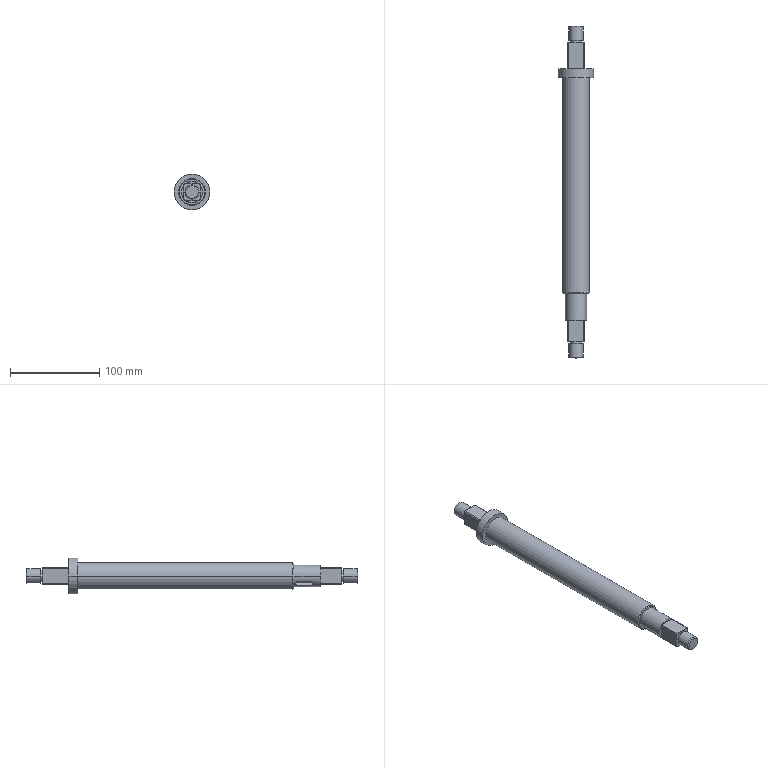Part | SolidWorks | features MirrorStock 1 | 1 solid | 50 faces | box 40 x 372 x 40 mm | volume 221068 mm3 | plane 24 | cylinder 20 | cone 6 | commonest cylinder face diameters 24 x6 13 x4 16 x4 6 x2 30 x2 40 x2
STEP:
#1=CARTESIAN_POINT('',(-7.,-186.,0.));
#2=VERTEX_POINT('',#1);
#3=CARTESIAN_POINT('',(7.,-186.,0.));
#4=VERTEX_POINT('',#3);
#5=CARTESIAN_POINT('',(0.,-186.,0.));
#6=DIRECTION('',(0.,1.,0.));
#7=DIRECTION('',(-1.,0.,0.));
#8=AXIS2_PLACEMENT_3D('',#5,#6,#7);
#9=CIRCLE('',#8,7.);
#10=EDGE_CURVE('',#2,#4,#9,.T.);
#11=ORIENTED_EDGE('',*,*,#10,.T.);
#12=CARTESIAN_POINT('',(8.,-185.,0.));
#13=VERTEX_POINT('',#12);
#14=CARTESIAN_POINT('',(7.,-186.,0.));
#15=DIRECTION('',(0.7071,0.7071,0.));
#16=VECTOR('',#15,1000.);
#17=LINE('',#14,#16);
#18=EDGE_CURVE('',#4,#13,#17,.T.);
#19=ORIENTED_EDGE('',*,*,#18,.T.);
#20=CARTESIAN_POINT('',(-8.,-185.,0.));
#21=VERTEX_POINT('',#20);
#22=CARTESIAN_POINT('',(0.,-185.,0.));
#23=DIRECTION('',(0.,-1.,0.));
#24=DIRECTION('',(-1.,0.,0.));
#25=AXIS2_PLACEMENT_3D('',#22,#23,#24);
#26=CIRCLE('',#25,8.);
#27=EDGE_CURVE('',#13,#21,#26,.T.);
#28=ORIENTED_EDGE('',*,*,#27,.T.);
#29=CARTESIAN_POINT('',(-7.,-186.,0.));
#30=DIRECTION('',(-0.7071,0.7071,0.));
#31=VECTOR('',#30,1000.);
#32=LINE('',#29,#31);
#33=EDGE_CURVE('',#2,#21,#32,.T.);
#34=ORIENTED_EDGE('',*,*,#33,.F.);
#35=EDGE_LOOP('',(#11,#19,#28,#34));
#36=FACE_OUTER_BOUND('',#35,.T.);
#37=CARTESIAN_POINT('',(0.,-186.,0.));
#38=DIRECTION('',(0.,1.,0.));
#39=DIRECTION('',(-1.,0.,0.));
#40=AXIS2_PLACEMENT_3D('',#37,#38,#39);
#41=CONICAL_SURFACE('',#40,7.,0.7854);
#42=ADVANCED_FACE('',(#36),#41,.T.);
#43=CARTESIAN_POINT('',(-14.,-114.,0.));
#44=VERTEX_POINT('',#43);
#45=CARTESIAN_POINT('',(14.,-114.,0.));
#46=VERTEX_POINT('',#45);
#47=CARTESIAN_POINT('',(0.,-114.,0.));
#48=DIRECTION('',(0.,1.,0.));
#49=DIRECTION('',(-1.,0.,0.));
#50=AXIS2_PLACEMENT_3D('',#47,#48,#49);
#51=CIRCLE('',#50,14.);
#52=EDGE_CURVE('',#44,#46,#51,.T.);
#53=ORIENTED_EDGE('',*,*,#52,.T.);
#54=CARTESIAN_POINT('',(15.,-113.,0.));
#55=VERTEX_POINT('',#54);
#56=CARTESIAN_POINT('',(14.,-114.,0.));
#57=DIRECTION('',(0.7071,0.7071,0.));
#58=VECTOR('',#57,1000.);
#59=LINE('',#56,#58);
#60=EDGE_CURVE('',#46,#55,#59,.T.);
#61=ORIENTED_EDGE('',*,*,#60,.T.);
#62=CARTESIAN_POINT('',(-15.,-113.,0.));
#63=VERTEX_POINT('',#62);
#64=CARTESIAN_POINT('',(0.,-113.,0.));
#65=DIRECTION('',(0.,-1.,0.));
#66=DIRECTION('',(-1.,0.,0.));
#67=AXIS2_PLACEMENT_3D('',#64,#65,#66);
#68=CIRCLE('',#67,15.);
#69=EDGE_CURVE('',#55,#63,#68,.T.);
#70=ORIENTED_EDGE('',*,*,#69,.T.);
#71=CARTESIAN_POINT('',(-14.,-114.,0.));
#72=DIRECTION('',(-0.7071,0.7071,0.));
#73=VECTOR('',#72,1000.);
#74=LINE('',#71,#73);
#75=EDGE_CURVE('',#44,#63,#74,.T.);
#76=ORIENTED_EDGE('',*,*,#75,.F.);
#77=EDGE_LOOP('',(#53,#61,#70,#76));
#78=FACE_OUTER_BOUND('',#77,.T.);
#79=CARTESIAN_POINT('',(0.,-114.,0.));
#80=DIRECTION('',(0.,1.,0.));
#81=DIRECTION('',(-1.,0.,0.));
#82=AXIS2_PLACEMENT_3D('',#79,#80,#81);
#83=CONICAL_SURFACE('',#82,14.,0.7854);
#84=ADVANCED_FACE('',(#78),#83,.T.);
#85=CARTESIAN_POINT('',(7.,186.,0.));
#86=VERTEX_POINT('',#85);
#87=CARTESIAN_POINT('',(-7.,186.,0.));
#88=VERTEX_POINT('',#87);
#89=CARTESIAN_POINT('',(0.,186.,0.));
#90=DIRECTION('',(0.,-1.,0.));
#91=DIRECTION('',(1.,0.,0.));
#92=AXIS2_PLACEMENT_3D('',#89,#90,#91);
#93=CIRCLE('',#92,7.);
#94=EDGE_CURVE('',#86,#88,#93,.T.);
#95=ORIENTED_EDGE('',*,*,#94,.T.);
#96=CARTESIAN_POINT('',(-8.,185.,0.));
#97=VERTEX_POINT('',#96);
#98=CARTESIAN_POINT('',(-8.,185.,0.));
#99=DIRECTION('',(-0.7071,-0.7071,0.));
#100=VECTOR('',#99,1000.);
#101=LINE('',#98,#100);
#102=EDGE_CURVE('',#88,#97,#101,.T.);
#103=ORIENTED_EDGE('',*,*,#102,.T.);
#104=CARTESIAN_POINT('',(8.,185.,0.));
#105=VERTEX_POINT('',#104);
#106=CARTESIAN_POINT('',(0.,185.,0.));
#107=DIRECTION('',(0.,1.,0.));
#108=DIRECTION('',(1.,0.,0.));
#109=AXIS2_PLACEMENT_3D('',#106,#107,#108);
#110=CIRCLE('',#109,8.);
#111=EDGE_CURVE('',#97,#105,#110,.T.);
#112=ORIENTED_EDGE('',*,*,#111,.T.);
#113=CARTESIAN_POINT('',(8.,185.,0.));
#114=DIRECTION('',(0.7071,-0.7071,0.));
#115=VECTOR('',#114,1000.);
#116=LINE('',#113,#115);
#117=EDGE_CURVE('',#86,#105,#116,.T.);
#118=ORIENTED_EDGE('',*,*,#117,.F.);
#119=EDGE_LOOP('',(#95,#103,#112,#118));
#120=FACE_OUTER_BOUND('',#119,.T.);
#121=CARTESIAN_POINT('',(0.,185.,0.));
#122=DIRECTION('',(0.,-1.,0.));
#123=DIRECTION('',(1.,0.,0.));
#124=AXIS2_PLACEMENT_3D('',#121,#122,#123);
#125=CONICAL_SURFACE('',#124,8.,0.7854);
#126=ADVANCED_FACE('',(#120),#125,.T.);
#127=CARTESIAN_POINT('',(-8.,-170.,0.));
#128=VERTEX_POINT('',#127);
#129=CARTESIAN_POINT('',(8.,-170.,0.));
#130=VERTEX_POINT('',#129);
#131=CARTESIAN_POINT('',(0.,-170.,0.));
#132=DIRECTION('',(0.,1.,0.));
#133=DIRECTION('',(1.,0.,0.));
#134=AXIS2_PLACEMENT_3D('',#131,#132,#133);
#135=CIRCLE('',#134,8.);
#136=EDGE_CURVE('',#128,#130,#135,.T.);
#137=ORIENTED_EDGE('',*,*,#136,.F.);
#138=CARTESIAN_POINT('',(-8.,-186.,0.));
#139=DIRECTION('',(0.,-1.,0.));
#140=VECTOR('',#139,1000.);
#141=LINE('',#138,#140);
#142=EDGE_CURVE('',#128,#21,#141,.T.);
#143=ORIENTED_EDGE('',*,*,#142,.T.);
#144=ORIENTED_EDGE('',*,*,#27,.F.);
#145=CARTESIAN_POINT('',(8.,-186.,0.));
#146=DIRECTION('',(0.,-1.,0.));
#147=VECTOR('',#146,1000.);
#148=LINE('',#145,#147);
#149=EDGE_CURVE('',#130,#13,#148,.T.);
#150=ORIENTED_EDGE('',*,*,#149,.F.);
#151=EDGE_LOOP('',(#137,#143,#144,#150));
#152=FACE_OUTER_BOUND('',#151,.T.);
#153=CARTESIAN_POINT('',(0.,-186.,0.));
#154=DIRECTION('',(0.,-1.,0.));
#155=DIRECTION('',(1.,0.,0.));
#156=AXIS2_PLACEMENT_3D('',#153,#154,#155);
#157=CYLINDRICAL_SURFACE('',#156,8.);
#158=ADVANCED_FACE('',(#152),#157,.T.);
#159=CARTESIAN_POINT('',(-6.5,-168.,0.));
#160=VERTEX_POINT('',#159);
#161=CARTESIAN_POINT('',(6.5,-168.,0.));
#162=VERTEX_POINT('',#161);
#163=CARTESIAN_POINT('',(0.,-168.,0.));
#164=DIRECTION('',(0.,1.,0.));
#165=DIRECTION('',(1.,0.,0.));
#166=AXIS2_PLACEMENT_3D('',#163,#164,#165);
#167=CIRCLE('',#166,6.5);
#168=EDGE_CURVE('',#160,#162,#167,.T.);
#169=ORIENTED_EDGE('',*,*,#168,.F.);
#170=CARTESIAN_POINT('',(-6.5,-170.,0.));
#171=VERTEX_POINT('',#170);
#172=CARTESIAN_POINT('',(-6.5,-186.,0.));
#173=DIRECTION('',(0.,-1.,0.));
#174=VECTOR('',#173,1000.);
#175=LINE('',#172,#174);
#176=EDGE_CURVE('',#160,#171,#175,.T.);
#177=ORIENTED_EDGE('',*,*,#176,.T.);
#178=CARTESIAN_POINT('',(6.5,-170.,0.));
#179=VERTEX_POINT('',#178);
#180=CARTESIAN_POINT('',(0.,-170.,0.));
#181=DIRECTION('',(0.,1.,0.));
#182=DIRECTION('',(1.,0.,0.));
#183=AXIS2_PLACEMENT_3D('',#180,#181,#182);
#184=CIRCLE('',#183,6.5);
#185=EDGE_CURVE('',#171,#179,#184,.T.);
#186=ORIENTED_EDGE('',*,*,#185,.T.);
#187=CARTESIAN_POINT('',(6.5,-186.,0.));
#188=DIRECTION('',(0.,-1.,0.));
#189=VECTOR('',#188,1000.);
#190=LINE('',#187,#189);
#191=EDGE_CURVE('',#162,#179,#190,.T.);
#192=ORIENTED_EDGE('',*,*,#191,.F.);
#193=EDGE_LOOP('',(#169,#177,#186,#192));
#194=FACE_OUTER_BOUND('',#193,.T.);
#195=CARTESIAN_POINT('',(0.,-186.,0.));
#196=DIRECTION('',(0.,-1.,0.));
#197=DIRECTION('',(1.,0.,0.));
#198=AXIS2_PLACEMENT_3D('',#195,#196,#197);
#199=CYLINDRICAL_SURFACE('',#198,6.5);
#200=ADVANCED_FACE('',(#194),#199,.T.);
#201=CARTESIAN_POINT('',(-15.,128.,0.));
#202=VERTEX_POINT('',#201);
#203=CARTESIAN_POINT('',(15.,128.,0.));
#204=VERTEX_POINT('',#203);
#205=CARTESIAN_POINT('',(0.,128.,0.));
#206=DIRECTION('',(0.,1.,0.));
#207=DIRECTION('',(1.,0.,0.));
#208=AXIS2_PLACEMENT_3D('',#205,#206,#207);
#209=CIRCLE('',#208,15.);
#210=EDGE_CURVE('',#202,#204,#209,.T.);
#211=ORIENTED_EDGE('',*,*,#210,.F.);
#212=CARTESIAN_POINT('',(-15.,-186.,0.));
#213=DIRECTION('',(0.,-1.,0.));
#214=VECTOR('',#213,1000.);
#215=LINE('',#212,#214);
#216=EDGE_CURVE('',#202,#63,#215,.T.);
#217=ORIENTED_EDGE('',*,*,#216,.T.);
#218=ORIENTED_EDGE('',*,*,#69,.F.);
#219=CARTESIAN_POINT('',(15.,-186.,0.));
#220=DIRECTION('',(0.,-1.,0.));
#221=VECTOR('',#220,1000.);
#222=LINE('',#219,#221);
#223=EDGE_CURVE('',#204,#55,#222,.T.);
#224=ORIENTED_EDGE('',*,*,#223,.F.);
#225=EDGE_LOOP('',(#211,#217,#218,#224));
#226=FACE_OUTER_BOUND('',#225,.T.);
#227=CARTESIAN_POINT('',(0.,-186.,0.));
#228=DIRECTION('',(0.,-1.,0.));
#229=DIRECTION('',(1.,0.,0.));
#230=AXIS2_PLACEMENT_3D('',#227,#228,#229);
#231=CYLINDRICAL_SURFACE('',#230,15.);
#232=ADVANCED_FACE('',(#226),#231,.T.);
#233=CARTESIAN_POINT('',(-20.,138.,0.));
#234=VERTEX_POINT('',#233);
#235=CARTESIAN_POINT('',(20.,138.,0.));
#236=VERTEX_POINT('',#235);
#237=CARTESIAN_POINT('',(0.,138.,0.));
#238=DIRECTION('',(0.,1.,0.));
#239=DIRECTION('',(1.,0.,0.));
#240=AXIS2_PLACEMENT_3D('',#237,#238,#239);
#241=CIRCLE('',#240,20.);
#242=EDGE_CURVE('',#234,#236,#241,.T.);
#243=ORIENTED_EDGE('',*,*,#242,.F.);
#244=CARTESIAN_POINT('',(-20.,128.,0.));
#245=VERTEX_POINT('',#244);
#246=CARTESIAN_POINT('',(-20.,-186.,0.));
#247=DIRECTION('',(0.,-1.,0.));
#248=VECTOR('',#247,1000.);
#249=LINE('',#246,#248);
#250=EDGE_CURVE('',#234,#245,#249,.T.);
#251=ORIENTED_EDGE('',*,*,#250,.T.);
#252=CARTESIAN_POINT('',(20.,128.,0.));
#253=VERTEX_POINT('',#252);
#254=CARTESIAN_POINT('',(0.,128.,0.));
#255=DIRECTION('',(0.,1.,0.));
#256=DIRECTION('',(1.,0.,0.));
#257=AXIS2_PLACEMENT_3D('',#254,#255,#256);
#258=CIRCLE('',#257,20.);
#259=EDGE_CURVE('',#245,#253,#258,.T.);
#260=ORIENTED_EDGE('',*,*,#259,.T.);
#261=CARTESIAN_POINT('',(20.,-186.,0.));
#262=DIRECTION('',(0.,-1.,0.));
#263=VECTOR('',#262,1000.);
#264=LINE('',#261,#263);
#265=EDGE_CURVE('',#236,#253,#264,.T.);
#266=ORIENTED_EDGE('',*,*,#265,.F.);
#267=EDGE_LOOP('',(#243,#251,#260,#266));
#268=FACE_OUTER_BOUND('',#267,.T.);
#269=CARTESIAN_POINT('',(0.,-186.,0.));
#270=DIRECTION('',(0.,-1.,0.));
#271=DIRECTION('',(1.,0.,0.));
#272=AXIS2_PLACEMENT_3D('',#269,#270,#271);
#273=CYLINDRICAL_SURFACE('',#272,20.);
#274=ADVANCED_FACE('',(#268),#273,.T.);
#275=CARTESIAN_POINT('',(-6.5,170.,0.));
#276=VERTEX_POINT('',#275);
#277=CARTESIAN_POINT('',(6.5,170.,0.));
#278=VERTEX_POINT('',#277);
#279=CARTESIAN_POINT('',(0.,170.,0.));
#280=DIRECTION('',(0.,1.,0.));
#281=DIRECTION('',(1.,0.,0.));
#282=AXIS2_PLACEMENT_3D('',#279,#280,#281);
#283=CIRCLE('',#282,6.5);
#284=EDGE_CURVE('',#276,#278,#283,.T.);
#285=ORIENTED_EDGE('',*,*,#284,.F.);
#286=CARTESIAN_POINT('',(-6.5,168.,0.));
#287=VERTEX_POINT('',#286);
#288=CARTESIAN_POINT('',(-6.5,-186.,0.));
#289=DIRECTION('',(0.,-1.,0.));
#290=VECTOR('',#289,1000.);
#291=LINE('',#288,#290);
#292=EDGE_CURVE('',#276,#287,#291,.T.);
#293=ORIENTED_EDGE('',*,*,#292,.T.);
#294=CARTESIAN_POINT('',(6.5,168.,0.));
#295=VERTEX_POINT('',#294);
#296=CARTESIAN_POINT('',(0.,168.,0.));
#297=DIRECTION('',(0.,1.,0.));
#298=DIRECTION('',(1.,0.,0.));
#299=AXIS2_PLACEMENT_3D('',#296,#297,#298);
#300=CIRCLE('',#299,6.5);
#301=EDGE_CURVE('',#287,#295,#300,.T.);
#302=ORIENTED_EDGE('',*,*,#301,.T.);
#303=CARTESIAN_POINT('',(6.5,-186.,0.));
#304=DIRECTION('',(0.,-1.,0.));
#305=VECTOR('',#304,1000.);
#306=LINE('',#303,#305);
#307=EDGE_CURVE('',#278,#295,#306,.T.);
#308=ORIENTED_EDGE('',*,*,#307,.F.);
#309=EDGE_LOOP('',(#285,#293,#302,#308));
#310=FACE_OUTER_BOUND('',#309,.T.);
#311=CARTESIAN_POINT('',(0.,-186.,0.));
#312=DIRECTION('',(0.,-1.,0.));
#313=DIRECTION('',(1.,0.,0.));
#314=AXIS2_PLACEMENT_3D('',#311,#312,#313);
#315=CYLINDRICAL_SURFACE('',#314,6.5);
#316=ADVANCED_FACE('',(#310),#315,.T.);
#317=ORIENTED_EDGE('',*,*,#111,.F.);
#318=CARTESIAN_POINT('',(-8.,170.,0.));
#319=VERTEX_POINT('',#318);
#320=CARTESIAN_POINT('',(-8.,-186.,0.));
#321=DIRECTION('',(0.,-1.,0.));
#322=VECTOR('',#321,1000.);
#323=LINE('',#320,#322);
#324=EDGE_CURVE('',#97,#319,#323,.T.);
#325=ORIENTED_EDGE('',*,*,#324,.T.);
#326=CARTESIAN_POINT('',(8.,170.,0.));
#327=VERTEX_POINT('',#326);
#328=CARTESIAN_POINT('',(0.,170.,0.));
#329=DIRECTION('',(0.,1.,0.));
#330=DIRECTION('',(1.,0.,0.));
#331=AXIS2_PLACEMENT_3D('',#328,#329,#330);
#332=CIRCLE('',#331,8.);
#333=EDGE_CURVE('',#319,#327,#332,.T.);
#334=ORIENTED_EDGE('',*,*,#333,.T.);
#335=CARTESIAN_POINT('',(8.,-186.,0.));
#336=DIRECTION('',(0.,-1.,0.));
#337=VECTOR('',#336,1000.);
#338=LINE('',#335,#337);
#339=EDGE_CURVE('',#105,#327,#338,.T.);
#340=ORIENTED_EDGE('',*,*,#339,.F.);
#341=EDGE_LOOP('',(#317,#325,#334,#340));
#342=FACE_OUTER_BOUND('',#341,.T.);
#343=CARTESIAN_POINT('',(0.,-186.,0.));
#344=DIRECTION('',(0.,-1.,0.));
#345=DIRECTION('',(1.,0.,0.));
#346=AXIS2_PLACEMENT_3D('',#343,#344,#345);
#347=CYLINDRICAL_SURFACE('',#346,8.);
#348=ADVANCED_FACE('',(#342),#347,.T.);
#349=CARTESIAN_POINT('',(-12.,-114.,0.));
#350=VERTEX_POINT('',#349);
#351=CARTESIAN_POINT('',(12.,-114.,0.));
#352=VERTEX_POINT('',#351);
#353=CARTESIAN_POINT('',(0.,-114.,0.));
#354=DIRECTION('',(0.,1.,0.));
#355=DIRECTION('',(1.,0.,0.));
#356=AXIS2_PLACEMENT_3D('',#353,#354,#355);
#357=CIRCLE('',#356,12.);
#358=EDGE_CURVE('',#350,#352,#357,.T.);
#359=ORIENTED_EDGE('',*,*,#358,.F.);
#360=CARTESIAN_POINT('',(-12.,-144.,0.));
#361=VERTEX_POINT('',#360);
#362=CARTESIAN_POINT('',(-12.,-186.,0.));
#363=DIRECTION('',(0.,-1.,0.));
#364=VECTOR('',#363,1000.);
#365=LINE('',#362,#364);
#366=EDGE_CURVE('',#350,#361,#365,.T.);
#367=ORIENTED_EDGE('',*,*,#366,.T.);
#368=CARTESIAN_POINT('',(-9.,-144.,7.937));
#369=VERTEX_POINT('',#368);
#370=CARTESIAN_POINT('',(0.,-144.,0.));
#371=DIRECTION('',(0.,1.,0.));
#372=DIRECTION('',(1.,0.,0.));
#373=AXIS2_PLACEMENT_3D('',#370,#371,#372);
#374=CIRCLE('',#373,12.);
#375=EDGE_CURVE('',#361,#369,#374,.T.);
#376=ORIENTED_EDGE('',*,*,#375,.T.);
#377=CARTESIAN_POINT('',(-9.,-168.,7.937));
#378=VERTEX_POINT('',#377);
#379=CARTESIAN_POINT('',(-9.,-186.,7.937));
#380=DIRECTION('',(0.,-1.,0.));
#381=VECTOR('',#380,1000.);
#382=LINE('',#379,#381);
#383=EDGE_CURVE('',#369,#378,#382,.T.);
#384=ORIENTED_EDGE('',*,*,#383,.T.);
#385=CARTESIAN_POINT('',(-7.937,-168.,9.));
#386=VERTEX_POINT('',#385);
#387=CARTESIAN_POINT('',(0.,-168.,0.));
#388=DIRECTION('',(0.,1.,0.));
#389=DIRECTION('',(1.,0.,0.));
#390=AXIS2_PLACEMENT_3D('',#387,#388,#389);
#391=CIRCLE('',#390,12.);
#392=EDGE_CURVE('',#378,#386,#391,.T.);
#393=ORIENTED_EDGE('',*,*,#392,.T.);
#394=CARTESIAN_POINT('',(-7.937,-144.,9.));
#395=VERTEX_POINT('',#394);
#396=CARTESIAN_POINT('',(-7.937,-186.,9.));
#397=DIRECTION('',(0.,1.,0.));
#398=VECTOR('',#397,1000.);
#399=LINE('',#396,#398);
#400=EDGE_CURVE('',#386,#395,#399,.T.);
#401=ORIENTED_EDGE('',*,*,#400,.T.);
#402=CARTESIAN_POINT('',(7.937,-144.,9.));
#403=VERTEX_POINT('',#402);
#404=CARTESIAN_POINT('',(0.,-144.,0.));
#405=DIRECTION('',(0.,1.,0.));
#406=DIRECTION('',(1.,0.,0.));
#407=AXIS2_PLACEMENT_3D('',#404,#405,#406);
#408=CIRCLE('',#407,12.);
#409=EDGE_CURVE('',#395,#403,#408,.T.);
#410=ORIENTED_EDGE('',*,*,#409,.T.);
#411=CARTESIAN_POINT('',(7.937,-168.,9.));
#412=VERTEX_POINT('',#411);
#413=CARTESIAN_POINT('',(7.937,-186.,9.));
#414=DIRECTION('',(0.,-1.,0.));
#415=VECTOR('',#414,1000.);
#416=LINE('',#413,#415);
#417=EDGE_CURVE('',#403,#412,#416,.T.);
#418=ORIENTED_EDGE('',*,*,#417,.T.);
#419=CARTESIAN_POINT('',(9.,-168.,7.937));
#420=VERTEX_POINT('',#419);
#421=CARTESIAN_POINT('',(0.,-168.,0.));
#422=DIRECTION('',(0.,1.,0.));
#423=DIRECTION('',(1.,0.,0.));
#424=AXIS2_PLACEMENT_3D('',#421,#422,#423);
#425=CIRCLE('',#424,12.);
#426=EDGE_CURVE('',#412,#420,#425,.T.);
#427=ORIENTED_EDGE('',*,*,#426,.T.);
#428=CARTESIAN_POINT('',(9.,-144.,7.937));
#429=VERTEX_POINT('',#428);
#430=CARTESIAN_POINT('',(9.,-186.,7.937));
#431=DIRECTION('',(0.,1.,0.));
#432=VECTOR('',#431,1000.);
#433=LINE('',#430,#432);
#434=EDGE_CURVE('',#420,#429,#433,.T.);
#435=ORIENTED_EDGE('',*,*,#434,.T.);
#436=CARTESIAN_POINT('',(12.,-144.,0.));
#437=VERTEX_POINT('',#436);
#438=CARTESIAN_POINT('',(0.,-144.,0.));
#439=DIRECTION('',(0.,1.,0.));
#440=DIRECTION('',(1.,0.,0.));
#441=AXIS2_PLACEMENT_3D('',#438,#439,#440);
#442=CIRCLE('',#441,12.);
#443=EDGE_CURVE('',#429,#437,#442,.T.);
#444=ORIENTED_EDGE('',*,*,#443,.T.);
#445=CARTESIAN_POINT('',(12.,-186.,0.));
#446=DIRECTION('',(0.,-1.,0.));
#447=VECTOR('',#446,1000.);
#448=LINE('',#445,#447);
#449=EDGE_CURVE('',#352,#437,#448,.T.);
#450=ORIENTED_EDGE('',*,*,#449,.F.);
#451=EDGE_LOOP('',(#359,#367,#376,#384,#393,#401,#410,#418,#427,#435,#444,#450));
#452=FACE_OUTER_BOUND('',#451,.T.);
#453=CARTESIAN_POINT('',(0.,-186.,0.));
#454=DIRECTION('',(0.,-1.,0.));
#455=DIRECTION('',(1.,0.,0.));
#456=AXIS2_PLACEMENT_3D('',#453,#454,#455);
#457=CYLINDRICAL_SURFACE('',#456,12.);
#458=ADVANCED_FACE('',(#452),#457,.T.);
#459=ORIENTED_EDGE('',*,*,#366,.F.);
#460=CARTESIAN_POINT('',(0.,-114.,0.));
#461=DIRECTION('',(0.,1.,0.));
#462=DIRECTION('',(1.,0.,0.));
#463=AXIS2_PLACEMENT_3D('',#460,#461,#462);
#464=CIRCLE('',#463,12.);
#465=EDGE_CURVE('',#352,#350,#464,.T.);
#466=ORIENTED_EDGE('',*,*,#465,.F.);
#467=ORIENTED_EDGE('',*,*,#449,.T.);
#468=CARTESIAN_POINT('',(9.,-144.,-7.937));
#469=VERTEX_POINT('',#468);
#470=CARTESIAN_POINT('',(0.,-144.,0.));
#471=DIRECTION('',(0.,1.,0.));
#472=DIRECTION('',(1.,0.,0.));
#473=AXIS2_PLACEMENT_3D('',#470,#471,#472);
#474=CIRCLE('',#473,12.);
#475=EDGE_CURVE('',#437,#469,#474,.T.);
#476=ORIENTED_EDGE('',*,*,#475,.T.);
#477=CARTESIAN_POINT('',(9.,-168.,-7.937));
#478=VERTEX_POINT('',#477);
#479=CARTESIAN_POINT('',(9.,-186.,-7.937));
#480=DIRECTION('',(0.,-1.,0.));
#481=VECTOR('',#480,1000.);
#482=LINE('',#479,#481);
#483=EDGE_CURVE('',#469,#478,#482,.T.);
#484=ORIENTED_EDGE('',*,*,#483,.T.);
#485=CARTESIAN_POINT('',(7.937,-168.,-9.));
#486=VERTEX_POINT('',#485);
#487=CARTESIAN_POINT('',(0.,-168.,0.));
#488=DIRECTION('',(0.,1.,0.));
#489=DIRECTION('',(1.,0.,0.));
#490=AXIS2_PLACEMENT_3D('',#487,#488,#489);
#491=CIRCLE('',#490,12.);
#492=EDGE_CURVE('',#478,#486,#491,.T.);
#493=ORIENTED_EDGE('',*,*,#492,.T.);
#494=CARTESIAN_POINT('',(7.937,-144.,-9.));
#495=VERTEX_POINT('',#494);
#496=CARTESIAN_POINT('',(7.937,-186.,-9.));
#497=DIRECTION('',(0.,1.,0.));
#498=VECTOR('',#497,1000.);
#499=LINE('',#496,#498);
#500=EDGE_CURVE('',#486,#495,#499,.T.);
#501=ORIENTED_EDGE('',*,*,#500,.T.);
#502=CARTESIAN_POINT('',(-7.937,-144.,-9.));
#503=VERTEX_POINT('',#502);
#504=CARTESIAN_POINT('',(0.,-144.,0.));
#505=DIRECTION('',(0.,1.,0.));
#506=DIRECTION('',(1.,0.,0.));
#507=AXIS2_PLACEMENT_3D('',#504,#505,#506);
#508=CIRCLE('',#507,12.);
#509=EDGE_CURVE('',#495,#503,#508,.T.);
#510=ORIENTED_EDGE('',*,*,#509,.T.);
#511=CARTESIAN_POINT('',(-7.937,-168.,-9.));
#512=VERTEX_POINT('',#511);
#513=CARTESIAN_POINT('',(-7.937,-186.,-9.));
#514=DIRECTION('',(0.,-1.,0.));
#515=VECTOR('',#514,1000.);
#516=LINE('',#513,#515);
#517=EDGE_CURVE('',#503,#512,#516,.T.);
#518=ORIENTED_EDGE('',*,*,#517,.T.);
#519=CARTESIAN_POINT('',(-9.,-168.,-7.937));
#520=VERTEX_POINT('',#519);
#521=CARTESIAN_POINT('',(0.,-168.,0.));
#522=DIRECTION('',(0.,1.,0.));
#523=DIRECTION('',(1.,0.,0.));
#524=AXIS2_PLACEMENT_3D('',#521,#522,#523);
#525=CIRCLE('',#524,12.);
#526=EDGE_CURVE('',#512,#520,#525,.T.);
#527=ORIENTED_EDGE('',*,*,#526,.T.);
#528=CARTESIAN_POINT('',(-9.,-144.,-7.937));
#529=VERTEX_POINT('',#528);
#530=CARTESIAN_POINT('',(-9.,-186.,-7.937));
#531=DIRECTION('',(0.,1.,0.));
#532=VECTOR('',#531,1000.);
#533=LINE('',#530,#532);
#534=EDGE_CURVE('',#520,#529,#533,.T.);
#535=ORIENTED_EDGE('',*,*,#534,.T.);
#536=CARTESIAN_POINT('',(0.,-144.,0.));
#537=DIRECTION('',(0.,1.,0.));
#538=DIRECTION('',(1.,0.,0.));
#539=AXIS2_PLACEMENT_3D('',#536,#537,#538);
#540=CIRCLE('',#539,12.);
#541=EDGE_CURVE('',#529,#361,#540,.T.);
#542=ORIENTED_EDGE('',*,*,#541,.T.);
#543=EDGE_LOOP('',(#459,#466,#467,#476,#484,#493,#501,#510,#518,#527,#535,#542));
#544=FACE_OUTER_BOUND('',#543,.T.);
#545=CARTESIAN_POINT('',(-6.095,-119.,-10.337));
#546=VERTEX_POINT('',#545);
#547=CARTESIAN_POINT('',(-10.337,-119.,-6.095));
#548=VERTEX_POINT('',#547);
#549=CARTESIAN_POINT('',(-6.095,-119.,-10.337));
#550=CARTESIAN_POINT('',(-6.095,-118.801,-10.337));
#551=CARTESIAN_POINT('',(-6.112,-118.605,-10.327));
#552=CARTESIAN_POINT('',(-6.18,-118.221,-10.286));
#553=CARTESIAN_POINT('',(-6.231,-118.03,-10.256));
#554=CARTESIAN_POINT('',(-6.363,-117.667,-10.174));
#555=CARTESIAN_POINT('',(-6.443,-117.495,-10.124));
#556=CARTESIAN_POINT('',(-6.63,-117.17,-10.003));
#557=CARTESIAN_POINT('',(-6.737,-117.016,-9.932));
#558=CARTESIAN_POINT('',(-6.967,-116.741,-9.772));
#559=CARTESIAN_POINT('',(-7.09,-116.617,-9.683));
#560=CARTESIAN_POINT('',(-7.354,-116.398,-9.484));
#561=CARTESIAN_POINT('',(-7.492,-116.305,-9.376));
#562=CARTESIAN_POINT('',(-7.771,-116.155,-9.145));
#563=CARTESIAN_POINT('',(-7.916,-116.097,-9.021));
#564=CARTESIAN_POINT('',(-8.203,-116.019,-8.761));
#565=CARTESIAN_POINT('',(-8.344,-116.,-8.626));
#566=CARTESIAN_POINT('',(-8.622,-116.,-8.348));
#567=CARTESIAN_POINT('',(-8.76,-116.019,-8.204));
#568=CARTESIAN_POINT('',(-9.019,-116.096,-7.918));
#569=CARTESIAN_POINT('',(-9.142,-116.153,-7.775));
#570=CARTESIAN_POINT('',(-9.491,-116.379,-7.352));
#571=CARTESIAN_POINT('',(-9.69,-116.6,-7.084));
#572=CARTESIAN_POINT('',(-9.932,-117.017,-6.736));
#573=CARTESIAN_POINT('',(-10.002,-117.167,-6.632));
#574=CARTESIAN_POINT('',(-10.123,-117.491,-6.445));
#575=CARTESIAN_POINT('',(-10.174,-117.667,-6.363));
#576=CARTESIAN_POINT('',(-10.255,-118.029,-6.232));
#577=CARTESIAN_POINT('',(-10.286,-118.216,-6.181));
#578=CARTESIAN_POINT('',(-10.327,-118.602,-6.112));
#579=CARTESIAN_POINT('',(-10.337,-118.801,-6.095));
#580=CARTESIAN_POINT('',(-10.337,-119.,-6.095));
#581=B_SPLINE_CURVE_WITH_KNOTS('',3,(#549,#550,#551,#552,#553,#554,#555,#556,#557,#558,#559,#560,#561,#562,#563,#564,#565,#566,#567,#568,#569,#570,#571,#572,#573,#574,#575,#576,#577,#578,#579,#580),.UNSPECIFIED.,.F.,.F.,(4,2,2,2,2,2,2,2,2,2,2,2,2,2,2,4),(0.,0.0005884,0.001177,0.001765,0.002353,0.002942,0.00353,0.004119,0.004707,0.005295,0.005884,0.00706,0.007649,0.008237,0.008826,0.009414),.UNSPECIFIED.);
#582=EDGE_CURVE('',#546,#548,#581,.T.);
#583=ORIENTED_EDGE('',*,*,#582,.T.);
#584=CARTESIAN_POINT('',(-10.337,-133.,-6.095));
#585=VERTEX_POINT('',#584);
#586=CARTESIAN_POINT('',(-10.337,-186.,-6.095));
#587=DIRECTION('',(0.,-1.,0.));
#588=VECTOR('',#587,1000.);
#589=LINE('',#586,#588);
#590=EDGE_CURVE('',#548,#585,#589,.T.);
#591=ORIENTED_EDGE('',*,*,#590,.T.);
#592=CARTESIAN_POINT('',(-6.095,-133.,-10.337));
#593=VERTEX_POINT('',#592);
#594=CARTESIAN_POINT('',(-10.337,-133.,-6.095));
#595=CARTESIAN_POINT('',(-10.337,-133.199,-6.095));
#596=CARTESIAN_POINT('',(-10.327,-133.395,-6.112));
#597=CARTESIAN_POINT('',(-10.286,-133.779,-6.18));
#598=CARTESIAN_POINT('',(-10.256,-133.97,-6.231));
#599=CARTESIAN_POINT('',(-10.174,-134.333,-6.363));
#600=CARTESIAN_POINT('',(-10.124,-134.505,-6.443));
#601=CARTESIAN_POINT('',(-10.003,-134.83,-6.63));
#602=CARTESIAN_POINT('',(-9.932,-134.984,-6.737));
#603=CARTESIAN_POINT('',(-9.772,-135.259,-6.967));
#604=CARTESIAN_POINT('',(-9.683,-135.383,-7.09));
#605=CARTESIAN_POINT('',(-9.484,-135.602,-7.354));
#606=CARTESIAN_POINT('',(-9.376,-135.695,-7.492));
#607=CARTESIAN_POINT('',(-9.145,-135.845,-7.771));
#608=CARTESIAN_POINT('',(-9.021,-135.903,-7.916));
#609=CARTESIAN_POINT('',(-8.761,-135.981,-8.203));
#610=CARTESIAN_POINT('',(-8.626,-136.,-8.344));
#611=CARTESIAN_POINT('',(-8.348,-136.,-8.622));
#612=CARTESIAN_POINT('',(-8.204,-135.981,-8.76));
#613=CARTESIAN_POINT('',(-7.918,-135.904,-9.019));
#614=CARTESIAN_POINT('',(-7.775,-135.847,-9.142));
#615=CARTESIAN_POINT('',(-7.352,-135.621,-9.491));
#616=CARTESIAN_POINT('',(-7.084,-135.4,-9.69));
#617=CARTESIAN_POINT('',(-6.736,-134.983,-9.932));
#618=CARTESIAN_POINT('',(-6.632,-134.833,-10.002));
#619=CARTESIAN_POINT('',(-6.445,-134.509,-10.123));
#620=CARTESIAN_POINT('',(-6.363,-134.333,-10.174));
#621=CARTESIAN_POINT('',(-6.232,-133.971,-10.255));
#622=CARTESIAN_POINT('',(-6.181,-133.784,-10.286));
#623=CARTESIAN_POINT('',(-6.112,-133.398,-10.327));
#624=CARTESIAN_POINT('',(-6.095,-133.199,-10.337));
#625=CARTESIAN_POINT('',(-6.095,-133.,-10.337));
#626=B_SPLINE_CURVE_WITH_KNOTS('',3,(#594,#595,#596,#597,#598,#599,#600,#601,#602,#603,#604,#605,#606,#607,#608,#609,#610,#611,#612,#613,#614,#615,#616,#617,#618,#619,#620,#621,#622,#623,#624,#625),.UNSPECIFIED.,.F.,.F.,(4,2,2,2,2,2,2,2,2,2,2,2,2,2,2,4),(0.,0.0005884,0.001177,0.001765,0.002353,0.002942,0.00353,0.004119,0.004707,0.005295,0.005884,0.00706,0.007649,0.008237,0.008826,0.009414),.UNSPECIFIED.);
#627=EDGE_CURVE('',#585,#593,#626,.T.);
#628=ORIENTED_EDGE('',*,*,#627,.T.);
#629=CARTESIAN_POINT('',(-6.095,-186.,-10.337));
#630=DIRECTION('',(0.,1.,0.));
#631=VECTOR('',#630,1000.);
#632=LINE('',#629,#631);
#633=EDGE_CURVE('',#593,#546,#632,.T.);
#634=ORIENTED_EDGE('',*,*,#633,.T.);
#635=EDGE_LOOP('',(#583,#591,#628,#634));
#636=FACE_BOUND('',#635,.T.);
#637=CARTESIAN_POINT('',(0.,-186.,0.));
#638=DIRECTION('',(0.,-1.,0.));
#639=DIRECTION('',(1.,0.,0.));
#640=AXIS2_PLACEMENT_3D('',#637,#638,#639);
#641=CYLINDRICAL_SURFACE('',#640,12.);
#642=ADVANCED_FACE('',(#544,#636),#641,.T.);
#643=CARTESIAN_POINT('',(0.,-168.,0.));
#644=DIRECTION('',(0.,1.,0.));
#645=DIRECTION('',(1.,0.,0.));
#646=AXIS2_PLACEMENT_3D('',#643,#644,#645);
#647=CIRCLE('',#646,6.5);
#648=EDGE_CURVE('',#162,#160,#647,.T.);
#649=ORIENTED_EDGE('',*,*,#648,.T.);
#650=ORIENTED_EDGE('',*,*,#168,.T.);
#651=EDGE_LOOP('',(#649,#650));
#652=FACE_BOUND('',#651,.T.);
#653=CARTESIAN_POINT('',(9.,-168.,0.));
#654=DIRECTION('',(0.,0.,1.));
#655=VECTOR('',#654,1000.);
#656=LINE('',#653,#655);
#657=EDGE_CURVE('',#478,#420,#656,.T.);
#658=ORIENTED_EDGE('',*,*,#657,.T.);
#659=ORIENTED_EDGE('',*,*,#426,.F.);
#660=CARTESIAN_POINT('',(-12.,-168.,9.));
#661=DIRECTION('',(-1.,0.,0.));
#662=VECTOR('',#661,1000.);
#663=LINE('',#660,#662);
#664=EDGE_CURVE('',#412,#386,#663,.T.);
#665=ORIENTED_EDGE('',*,*,#664,.T.);
#666=ORIENTED_EDGE('',*,*,#392,.F.);
#667=CARTESIAN_POINT('',(-9.,-168.,0.));
#668=DIRECTION('',(0.,0.,-1.));
#669=VECTOR('',#668,1000.);
#670=LINE('',#667,#669);
#671=EDGE_CURVE('',#378,#520,#670,.T.);
#672=ORIENTED_EDGE('',*,*,#671,.T.);
#673=ORIENTED_EDGE('',*,*,#526,.F.);
#674=CARTESIAN_POINT('',(-12.,-168.,-9.));
#675=DIRECTION('',(1.,0.,0.));
#676=VECTOR('',#675,1000.);
#677=LINE('',#674,#676);
#678=EDGE_CURVE('',#512,#486,#677,.T.);
#679=ORIENTED_EDGE('',*,*,#678,.T.);
#680=ORIENTED_EDGE('',*,*,#492,.F.);
#681=EDGE_LOOP('',(#658,#659,#665,#666,#672,#673,#679,#680));
#682=FACE_OUTER_BOUND('',#681,.T.);
#683=CARTESIAN_POINT('',(-12.,-168.,0.));
#684=DIRECTION('',(0.,1.,0.));
#685=DIRECTION('',(-1.,0.,0.));
#686=AXIS2_PLACEMENT_3D('',#683,#684,#685);
#687=PLANE('',#686);
#688=ADVANCED_FACE('',(#652,#682),#687,.F.);
#689=CARTESIAN_POINT('',(0.,168.,0.));
#690=DIRECTION('',(0.,1.,0.));
#691=DIRECTION('',(1.,0.,0.));
#692=AXIS2_PLACEMENT_3D('',#689,#690,#691);
#693=CIRCLE('',#692,6.5);
#694=EDGE_CURVE('',#295,#287,#693,.T.);
#695=ORIENTED_EDGE('',*,*,#694,.F.);
#696=ORIENTED_EDGE('',*,*,#301,.F.);
#697=EDGE_LOOP('',(#695,#696));
#698=FACE_BOUND('',#697,.T.);
#699=CARTESIAN_POINT('',(-9.,168.,7.937));
#700=VERTEX_POINT('',#699);
#701=CARTESIAN_POINT('',(-9.,168.,-7.937));
#702=VERTEX_POINT('',#701);
#703=CARTESIAN_POINT('',(-9.,168.,-9.));
#704=DIRECTION('',(0.,0.,-1.));
#705=VECTOR('',#704,1000.);
#706=LINE('',#703,#705);
#707=EDGE_CURVE('',#700,#702,#706,.T.);
#708=ORIENTED_EDGE('',*,*,#707,.F.);
#709=CARTESIAN_POINT('',(-7.937,168.,9.));
#710=VERTEX_POINT('',#709);
#711=CARTESIAN_POINT('',(0.,168.,0.));
#712=DIRECTION('',(0.,1.,0.));
#713=DIRECTION('',(1.,0.,0.));
#714=AXIS2_PLACEMENT_3D('',#711,#712,#713);
#715=CIRCLE('',#714,12.);
#716=EDGE_CURVE('',#700,#710,#715,.T.);
#717=ORIENTED_EDGE('',*,*,#716,.T.);
#718=CARTESIAN_POINT('',(7.937,168.,9.));
#719=VERTEX_POINT('',#718);
#720=CARTESIAN_POINT('',(9.,168.,9.));
#721=DIRECTION('',(-1.,0.,0.));
#722=VECTOR('',#721,1000.);
#723=LINE('',#720,#722);
#724=EDGE_CURVE('',#719,#710,#723,.T.);
#725=ORIENTED_EDGE('',*,*,#724,.F.);
#726=CARTESIAN_POINT('',(9.,168.,7.937));
#727=VERTEX_POINT('',#726);
#728=CARTESIAN_POINT('',(0.,168.,0.));
#729=DIRECTION('',(0.,1.,0.));
#730=DIRECTION('',(1.,0.,0.));
#731=AXIS2_PLACEMENT_3D('',#728,#729,#730);
#732=CIRCLE('',#731,12.);
#733=EDGE_CURVE('',#719,#727,#732,.T.);
#734=ORIENTED_EDGE('',*,*,#733,.T.);
#735=CARTESIAN_POINT('',(9.,168.,-7.937));
#736=VERTEX_POINT('',#735);
#737=CARTESIAN_POINT('',(9.,168.,-9.));
#738=DIRECTION('',(0.,0.,1.));
#739=VECTOR('',#738,1000.);
#740=LINE('',#737,#739);
#741=EDGE_CURVE('',#736,#727,#740,.T.);
#742=ORIENTED_EDGE('',*,*,#741,.F.);
#743=CARTESIAN_POINT('',(7.937,168.,-9.));
#744=VERTEX_POINT('',#743);
#745=CARTESIAN_POINT('',(0.,168.,0.));
#746=DIRECTION('',(0.,1.,0.));
#747=DIRECTION('',(1.,0.,0.));
#748=AXIS2_PLACEMENT_3D('',#745,#746,#747);
#749=CIRCLE('',#748,12.);
#750=EDGE_CURVE('',#736,#744,#749,.T.);
#751=ORIENTED_EDGE('',*,*,#750,.T.);
#752=CARTESIAN_POINT('',(-7.937,168.,-9.));
#753=VERTEX_POINT('',#752);
#754=CARTESIAN_POINT('',(9.,168.,-9.));
#755=DIRECTION('',(1.,0.,0.));
#756=VECTOR('',#755,1000.);
#757=LINE('',#754,#756);
#758=EDGE_CURVE('',#753,#744,#757,.T.);
#759=ORIENTED_EDGE('',*,*,#758,.F.);
#760=CARTESIAN_POINT('',(0.,168.,0.));
#761=DIRECTION('',(0.,1.,0.));
#762=DIRECTION('',(1.,0.,0.));
#763=AXIS2_PLACEMENT_3D('',#760,#761,#762);
#764=CIRCLE('',#763,12.);
#765=EDGE_CURVE('',#753,#702,#764,.T.);
#766=ORIENTED_EDGE('',*,*,#765,.T.);
#767=EDGE_LOOP('',(#708,#717,#725,#734,#742,#751,#759,#766));
#768=FACE_OUTER_BOUND('',#767,.T.);
#769=CARTESIAN_POINT('',(-6.5,168.,0.));
#770=DIRECTION('',(0.,-1.,0.));
#771=DIRECTION('',(1.,0.,0.));
#772=AXIS2_PLACEMENT_3D('',#769,#770,#771);
#773=PLANE('',#772);
#774=ADVANCED_FACE('',(#698,#768),#773,.F.);
#775=CARTESIAN_POINT('',(-9.,138.,7.937));
#776=VERTEX_POINT('',#775);
#777=CARTESIAN_POINT('',(-9.,-186.,7.937));
#778=DIRECTION('',(0.,-1.,0.));
#779=VECTOR('',#778,1000.);
#780=LINE('',#777,#779);
#781=EDGE_CURVE('',#700,#776,#780,.T.);
#782=ORIENTED_EDGE('',*,*,#781,.T.);
#783=CARTESIAN_POINT('',(-7.937,138.,9.));
#784=VERTEX_POINT('',#783);
#785=CARTESIAN_POINT('',(0.,138.,0.));
#786=DIRECTION('',(0.,1.,0.));
#787=DIRECTION('',(1.,0.,0.));
#788=AXIS2_PLACEMENT_3D('',#785,#786,#787);
#789=CIRCLE('',#788,12.);
#790=EDGE_CURVE('',#776,#784,#789,.T.);
#791=ORIENTED_EDGE('',*,*,#790,.T.);
#792=CARTESIAN_POINT('',(-7.937,-186.,9.));
#793=DIRECTION('',(0.,1.,0.));
#794=VECTOR('',#793,1000.);
#795=LINE('',#792,#794);
#796=EDGE_CURVE('',#784,#710,#795,.T.);
#797=ORIENTED_EDGE('',*,*,#796,.T.);
#798=ORIENTED_EDGE('',*,*,#716,.F.);
#799=EDGE_LOOP('',(#782,#791,#797,#798));
#800=FACE_OUTER_BOUND('',#799,.T.);
#801=CARTESIAN_POINT('',(0.,-186.,0.));
#802=DIRECTION('',(0.,-1.,0.));
#803=DIRECTION('',(1.,0.,0.));
#804=AXIS2_PLACEMENT_3D('',#801,#802,#803);
#805=CYLINDRICAL_SURFACE('',#804,12.);
#806=ADVANCED_FACE('',(#800),#805,.T.);
#807=CARTESIAN_POINT('',(-9.,138.,-7.937));
#808=VERTEX_POINT('',#807);
#809=CARTESIAN_POINT('',(-9.,-186.,-7.937));
#810=DIRECTION('',(0.,1.,0.));
#811=VECTOR('',#810,1000.);
#812=LINE('',#809,#811);
#813=EDGE_CURVE('',#808,#702,#812,.T.);
#814=ORIENTED_EDGE('',*,*,#813,.T.);
#815=ORIENTED_EDGE('',*,*,#765,.F.);
#816=CARTESIAN_POINT('',(-7.937,138.,-9.));
#817=VERTEX_POINT('',#816);
#818=CARTESIAN_POINT('',(-7.937,-186.,-9.));
#819=DIRECTION('',(0.,-1.,0.));
#820=VECTOR('',#819,1000.);
#821=LINE('',#818,#820);
#822=EDGE_CURVE('',#753,#817,#821,.T.);
#823=ORIENTED_EDGE('',*,*,#822,.T.);
#824=CARTESIAN_POINT('',(0.,138.,0.));
#825=DIRECTION('',(0.,1.,0.));
#826=DIRECTION('',(1.,0.,0.));
#827=AXIS2_PLACEMENT_3D('',#824,#825,#826);
#828=CIRCLE('',#827,12.);
#829=EDGE_CURVE('',#817,#808,#828,.T.);
#830=ORIENTED_EDGE('',*,*,#829,.T.);
#831=EDGE_LOOP('',(#814,#815,#823,#830));
#832=FACE_OUTER_BOUND('',#831,.T.);
#833=CARTESIAN_POINT('',(0.,-186.,0.));
#834=DIRECTION('',(0.,-1.,0.));
#835=DIRECTION('',(1.,0.,0.));
#836=AXIS2_PLACEMENT_3D('',#833,#834,#835);
#837=CYLINDRICAL_SURFACE('',#836,12.);
#838=ADVANCED_FACE('',(#832),#837,.T.);
#839=CARTESIAN_POINT('',(7.937,138.,9.));
#840=VERTEX_POINT('',#839);
#841=CARTESIAN_POINT('',(7.937,-186.,9.));
#842=DIRECTION('',(0.,-1.,0.));
#843=VECTOR('',#842,1000.);
#844=LINE('',#841,#843);
#845=EDGE_CURVE('',#719,#840,#844,.T.);
#846=ORIENTED_EDGE('',*,*,#845,.T.);
#847=CARTESIAN_POINT('',(9.,138.,7.937));
#848=VERTEX_POINT('',#847);
#849=CARTESIAN_POINT('',(0.,138.,0.));
#850=DIRECTION('',(0.,1.,0.));
#851=DIRECTION('',(1.,0.,0.));
#852=AXIS2_PLACEMENT_3D('',#849,#850,#851);
#853=CIRCLE('',#852,12.);
#854=EDGE_CURVE('',#840,#848,#853,.T.);
#855=ORIENTED_EDGE('',*,*,#854,.T.);
#856=CARTESIAN_POINT('',(9.,-186.,7.937));
#857=DIRECTION('',(0.,1.,0.));
#858=VECTOR('',#857,1000.);
#859=LINE('',#856,#858);
#860=EDGE_CURVE('',#848,#727,#859,.T.);
#861=ORIENTED_EDGE('',*,*,#860,.T.);
#862=ORIENTED_EDGE('',*,*,#733,.F.);
#863=EDGE_LOOP('',(#846,#855,#861,#862));
#864=FACE_OUTER_BOUND('',#863,.T.);
#865=CARTESIAN_POINT('',(0.,-186.,0.));
#866=DIRECTION('',(0.,-1.,0.));
#867=DIRECTION('',(1.,0.,0.));
#868=AXIS2_PLACEMENT_3D('',#865,#866,#867);
#869=CYLINDRICAL_SURFACE('',#868,12.);
#870=ADVANCED_FACE('',(#864),#869,.T.);
#871=CARTESIAN_POINT('',(9.,138.,-7.937));
#872=VERTEX_POINT('',#871);
#873=CARTESIAN_POINT('',(9.,-186.,-7.937));
#874=DIRECTION('',(0.,-1.,0.));
#875=VECTOR('',#874,1000.);
#876=LINE('',#873,#875);
#877=EDGE_CURVE('',#736,#872,#876,.T.);
#878=ORIENTED_EDGE('',*,*,#877,.T.);
#879=CARTESIAN_POINT('',(7.937,138.,-9.));
#880=VERTEX_POINT('',#879);
#881=CARTESIAN_POINT('',(0.,138.,0.));
#882=DIRECTION('',(0.,1.,0.));
#883=DIRECTION('',(1.,0.,0.));
#884=AXIS2_PLACEMENT_3D('',#881,#882,#883);
#885=CIRCLE('',#884,12.);
#886=EDGE_CURVE('',#872,#880,#885,.T.);
#887=ORIENTED_EDGE('',*,*,#886,.T.);
#888=CARTESIAN_POINT('',(7.937,-186.,-9.));
#889=DIRECTION('',(0.,1.,0.));
#890=VECTOR('',#889,1000.);
#891=LINE('',#888,#890);
#892=EDGE_CURVE('',#880,#744,#891,.T.);
#893=ORIENTED_EDGE('',*,*,#892,.T.);
#894=ORIENTED_EDGE('',*,*,#750,.F.);
#895=EDGE_LOOP('',(#878,#887,#893,#894));
#896=FACE_OUTER_BOUND('',#895,.T.);
#897=CARTESIAN_POINT('',(0.,-186.,0.));
#898=DIRECTION('',(0.,-1.,0.));
#899=DIRECTION('',(1.,0.,0.));
#900=AXIS2_PLACEMENT_3D('',#897,#898,#899);
#901=CYLINDRICAL_SURFACE('',#900,12.);
#902=ADVANCED_FACE('',(#896),#901,.T.);
#903=ORIENTED_EDGE('',*,*,#94,.F.);
#904=CARTESIAN_POINT('',(0.,186.,0.));
#905=DIRECTION('',(0.,-1.,0.));
#906=DIRECTION('',(1.,0.,0.));
#907=AXIS2_PLACEMENT_3D('',#904,#905,#906);
#908=CIRCLE('',#907,7.);
#909=EDGE_CURVE('',#88,#86,#908,.T.);
#910=ORIENTED_EDGE('',*,*,#909,.F.);
#911=EDGE_LOOP('',(#903,#910));
#912=FACE_OUTER_BOUND('',#911,.T.);
#913=CARTESIAN_POINT('',(0.,186.,0.));
#914=DIRECTION('',(0.,-1.,0.));
#915=DIRECTION('',(1.,0.,0.));
#916=AXIS2_PLACEMENT_3D('',#913,#914,#915);
#917=PLANE('',#916);
#918=ADVANCED_FACE('',(#912),#917,.F.);
#919=ORIENTED_EDGE('',*,*,#324,.F.);
#920=CARTESIAN_POINT('',(0.,185.,0.));
#921=DIRECTION('',(0.,1.,0.));
#922=DIRECTION('',(1.,0.,0.));
#923=AXIS2_PLACEMENT_3D('',#920,#921,#922);
#924=CIRCLE('',#923,8.);
#925=EDGE_CURVE('',#105,#97,#924,.T.);
#926=ORIENTED_EDGE('',*,*,#925,.F.);
#927=ORIENTED_EDGE('',*,*,#339,.T.);
#928=CARTESIAN_POINT('',(0.,170.,0.));
#929=DIRECTION('',(0.,1.,0.));
#930=DIRECTION('',(1.,0.,0.));
#931=AXIS2_PLACEMENT_3D('',#928,#929,#930);
#932=CIRCLE('',#931,8.);
#933=EDGE_CURVE('',#327,#319,#932,.T.);
#934=ORIENTED_EDGE('',*,*,#933,.T.);
#935=EDGE_LOOP('',(#919,#926,#927,#934));
#936=FACE_OUTER_BOUND('',#935,.T.);
#937=CARTESIAN_POINT('',(0.,-186.,0.));
#938=DIRECTION('',(0.,-1.,0.));
#939=DIRECTION('',(1.,0.,0.));
#940=AXIS2_PLACEMENT_3D('',#937,#938,#939);
#941=CYLINDRICAL_SURFACE('',#940,8.);
#942=ADVANCED_FACE('',(#936),#941,.T.);
#943=CARTESIAN_POINT('',(0.,170.,0.));
#944=DIRECTION('',(0.,1.,0.));
#945=DIRECTION('',(1.,0.,0.));
#946=AXIS2_PLACEMENT_3D('',#943,#944,#945);
#947=CIRCLE('',#946,6.5);
#948=EDGE_CURVE('',#278,#276,#947,.T.);
#949=ORIENTED_EDGE('',*,*,#948,.T.);
#950=ORIENTED_EDGE('',*,*,#284,.T.);
#951=EDGE_LOOP('',(#949,#950));
#952=FACE_BOUND('',#951,.T.);
#953=ORIENTED_EDGE('',*,*,#933,.F.);
#954=ORIENTED_EDGE('',*,*,#333,.F.);
#955=EDGE_LOOP('',(#953,#954));
#956=FACE_OUTER_BOUND('',#955,.T.);
#957=CARTESIAN_POINT('',(-8.,170.,0.));
#958=DIRECTION('',(0.,1.,0.));
#959=DIRECTION('',(-1.,0.,0.));
#960=AXIS2_PLACEMENT_3D('',#957,#958,#959);
#961=PLANE('',#960);
#962=ADVANCED_FACE('',(#952,#956),#961,.F.);
#963=ORIENTED_EDGE('',*,*,#292,.F.);
#964=ORIENTED_EDGE('',*,*,#948,.F.);
#965=ORIENTED_EDGE('',*,*,#307,.T.);
#966=ORIENTED_EDGE('',*,*,#694,.T.);
#967=EDGE_LOOP('',(#963,#964,#965,#966));
#968=FACE_OUTER_BOUND('',#967,.T.);
#969=CARTESIAN_POINT('',(0.,-186.,0.));
#970=DIRECTION('',(0.,-1.,0.));
#971=DIRECTION('',(1.,0.,0.));
#972=AXIS2_PLACEMENT_3D('',#969,#970,#971);
#973=CYLINDRICAL_SURFACE('',#972,6.5);
#974=ADVANCED_FACE('',(#968),#973,.T.);
#975=ORIENTED_EDGE('',*,*,#829,.F.);
#976=CARTESIAN_POINT('',(9.,138.,-9.));
#977=DIRECTION('',(1.,0.,0.));
#978=VECTOR('',#977,1000.);
#979=LINE('',#976,#978);
#980=EDGE_CURVE('',#817,#880,#979,.T.);
#981=ORIENTED_EDGE('',*,*,#980,.T.);
#982=ORIENTED_EDGE('',*,*,#886,.F.);
#983=CARTESIAN_POINT('',(9.,138.,-9.));
#984=DIRECTION('',(0.,0.,1.));
#985=VECTOR('',#984,1000.);
#986=LINE('',#983,#985);
#987=EDGE_CURVE('',#872,#848,#986,.T.);
#988=ORIENTED_EDGE('',*,*,#987,.T.);
#989=ORIENTED_EDGE('',*,*,#854,.F.);
#990=CARTESIAN_POINT('',(9.,138.,9.));
#991=DIRECTION('',(-1.,0.,0.));
#992=VECTOR('',#991,1000.);
#993=LINE('',#990,#992);
#994=EDGE_CURVE('',#840,#784,#993,.T.);
#995=ORIENTED_EDGE('',*,*,#994,.T.);
#996=ORIENTED_EDGE('',*,*,#790,.F.);
#997=CARTESIAN_POINT('',(-9.,138.,-9.));
#998=DIRECTION('',(0.,0.,-1.));
#999=VECTOR('',#998,1000.);
#1000=LINE('',#997,#999);
#1001=EDGE_CURVE('',#776,#808,#1000,.T.);
#1002=ORIENTED_EDGE('',*,*,#1001,.T.);
#1003=EDGE_LOOP('',(#975,#981,#982,#988,#989,#995,#996,#1002));
#1004=FACE_BOUND('',#1003,.T.);
#1005=CARTESIAN_POINT('',(0.,138.,0.));
#1006=DIRECTION('',(0.,1.,0.));
#1007=DIRECTION('',(1.,0.,0.));
#1008=AXIS2_PLACEMENT_3D('',#1005,#1006,#1007);
#1009=CIRCLE('',#1008,20.);
#1010=EDGE_CURVE('',#236,#234,#1009,.T.);
#1011=ORIENTED_EDGE('',*,*,#1010,.T.);
#1012=ORIENTED_EDGE('',*,*,#242,.T.);
#1013=EDGE_LOOP('',(#1011,#1012));
#1014=FACE_OUTER_BOUND('',#1013,.T.);
#1015=CARTESIAN_POINT('',(-12.,138.,0.));
#1016=DIRECTION('',(0.,-1.,0.));
#1017=DIRECTION('',(1.,0.,0.));
#1018=AXIS2_PLACEMENT_3D('',#1015,#1016,#1017);
#1019=PLANE('',#1018);
#1020=ADVANCED_FACE('',(#1004,#1014),#1019,.F.);
#1021=ORIENTED_EDGE('',*,*,#250,.F.);
#1022=ORIENTED_EDGE('',*,*,#1010,.F.);
#1023=ORIENTED_EDGE('',*,*,#265,.T.);
#1024=CARTESIAN_POINT('',(0.,128.,0.));
#1025=DIRECTION('',(0.,1.,0.));
#1026=DIRECTION('',(1.,0.,0.));
#1027=AXIS2_PLACEMENT_3D('',#1024,#1025,#1026);
#1028=CIRCLE('',#1027,20.);
#1029=EDGE_CURVE('',#253,#245,#1028,.T.);
#1030=ORIENTED_EDGE('',*,*,#1029,.T.);
#1031=EDGE_LOOP('',(#1021,#1022,#1023,#1030));
#1032=FACE_OUTER_BOUND('',#1031,.T.);
#1033=CARTESIAN_POINT('',(0.,-186.,0.));
#1034=DIRECTION('',(0.,-1.,0.));
#1035=DIRECTION('',(1.,0.,0.));
#1036=AXIS2_PLACEMENT_3D('',#1033,#1034,#1035);
#1037=CYLINDRICAL_SURFACE('',#1036,20.);
#1038=ADVANCED_FACE('',(#1032),#1037,.T.);
#1039=CARTESIAN_POINT('',(0.,128.,0.));
#1040=DIRECTION('',(0.,1.,0.));
#1041=DIRECTION('',(1.,0.,0.));
#1042=AXIS2_PLACEMENT_3D('',#1039,#1040,#1041);
#1043=CIRCLE('',#1042,15.);
#1044=EDGE_CURVE('',#204,#202,#1043,.T.);
#1045=ORIENTED_EDGE('',*,*,#1044,.T.);
#1046=ORIENTED_EDGE('',*,*,#210,.T.);
#1047=EDGE_LOOP('',(#1045,#1046));
#1048=FACE_BOUND('',#1047,.T.);
#1049=ORIENTED_EDGE('',*,*,#1029,.F.);
#1050=ORIENTED_EDGE('',*,*,#259,.F.);
#1051=EDGE_LOOP('',(#1049,#1050));
#1052=FACE_OUTER_BOUND('',#1051,.T.);
#1053=CARTESIAN_POINT('',(-20.,128.,0.));
#1054=DIRECTION('',(0.,1.,0.));
#1055=DIRECTION('',(-1.,0.,0.));
#1056=AXIS2_PLACEMENT_3D('',#1053,#1054,#1055);
#1057=PLANE('',#1056);
#1058=ADVANCED_FACE('',(#1048,#1052),#1057,.F.);
#1059=ORIENTED_EDGE('',*,*,#216,.F.);
#1060=ORIENTED_EDGE('',*,*,#1044,.F.);
#1061=ORIENTED_EDGE('',*,*,#223,.T.);
#1062=CARTESIAN_POINT('',(0.,-113.,0.));
#1063=DIRECTION('',(0.,-1.,0.));
#1064=DIRECTION('',(-1.,0.,0.));
#1065=AXIS2_PLACEMENT_3D('',#1062,#1063,#1064);
#1066=CIRCLE('',#1065,15.);
#1067=EDGE_CURVE('',#63,#55,#1066,.T.);
#1068=ORIENTED_EDGE('',*,*,#1067,.F.);
#1069=EDGE_LOOP('',(#1059,#1060,#1061,#1068));
#1070=FACE_OUTER_BOUND('',#1069,.T.);
#1071=CARTESIAN_POINT('',(0.,-186.,0.));
#1072=DIRECTION('',(0.,-1.,0.));
#1073=DIRECTION('',(1.,0.,0.));
#1074=AXIS2_PLACEMENT_3D('',#1071,#1072,#1073);
#1075=CYLINDRICAL_SURFACE('',#1074,15.);
#1076=ADVANCED_FACE('',(#1070),#1075,.T.);
#1077=ORIENTED_EDGE('',*,*,#52,.F.);
#1078=CARTESIAN_POINT('',(0.,-114.,0.));
#1079=DIRECTION('',(0.,1.,0.));
#1080=DIRECTION('',(-1.,0.,0.));
#1081=AXIS2_PLACEMENT_3D('',#1078,#1079,#1080);
#1082=CIRCLE('',#1081,14.);
#1083=EDGE_CURVE('',#46,#44,#1082,.T.);
#1084=ORIENTED_EDGE('',*,*,#1083,.F.);
#1085=EDGE_LOOP('',(#1077,#1084));
#1086=FACE_OUTER_BOUND('',#1085,.T.);
#1087=ORIENTED_EDGE('',*,*,#465,.T.);
#1088=ORIENTED_EDGE('',*,*,#358,.T.);
#1089=EDGE_LOOP('',(#1087,#1088));
#1090=FACE_BOUND('',#1089,.T.);
#1091=CARTESIAN_POINT('',(-15.,-114.,0.));
#1092=DIRECTION('',(0.,1.,0.));
#1093=DIRECTION('',(-1.,0.,0.));
#1094=AXIS2_PLACEMENT_3D('',#1091,#1092,#1093);
#1095=PLANE('',#1094);
#1096=ADVANCED_FACE('',(#1086,#1090),#1095,.F.);
#1097=ORIENTED_EDGE('',*,*,#176,.F.);
#1098=ORIENTED_EDGE('',*,*,#648,.F.);
#1099=ORIENTED_EDGE('',*,*,#191,.T.);
#1100=CARTESIAN_POINT('',(0.,-170.,0.));
#1101=DIRECTION('',(0.,1.,0.));
#1102=DIRECTION('',(1.,0.,0.));
#1103=AXIS2_PLACEMENT_3D('',#1100,#1101,#1102);
#1104=CIRCLE('',#1103,6.5);
#1105=EDGE_CURVE('',#179,#171,#1104,.T.);
#1106=ORIENTED_EDGE('',*,*,#1105,.T.);
#1107=EDGE_LOOP('',(#1097,#1098,#1099,#1106));
#1108=FACE_OUTER_BOUND('',#1107,.T.);
#1109=CARTESIAN_POINT('',(0.,-186.,0.));
#1110=DIRECTION('',(0.,-1.,0.));
#1111=DIRECTION('',(1.,0.,0.));
#1112=AXIS2_PLACEMENT_3D('',#1109,#1110,#1111);
#1113=CYLINDRICAL_SURFACE('',#1112,6.5);
#1114=ADVANCED_FACE('',(#1108),#1113,.T.);
#1115=CARTESIAN_POINT('',(0.,-170.,0.));
#1116=DIRECTION('',(0.,1.,0.));
#1117=DIRECTION('',(1.,0.,0.));
#1118=AXIS2_PLACEMENT_3D('',#1115,#1116,#1117);
#1119=CIRCLE('',#1118,8.);
#1120=EDGE_CURVE('',#130,#128,#1119,.T.);
#1121=ORIENTED_EDGE('',*,*,#1120,.T.);
#1122=ORIENTED_EDGE('',*,*,#136,.T.);
#1123=EDGE_LOOP('',(#1121,#1122));
#1124=FACE_OUTER_BOUND('',#1123,.T.);
#1125=ORIENTED_EDGE('',*,*,#1105,.F.);
#1126=ORIENTED_EDGE('',*,*,#185,.F.);
#1127=EDGE_LOOP('',(#1125,#1126));
#1128=FACE_BOUND('',#1127,.T.);
#1129=CARTESIAN_POINT('',(-6.5,-170.,0.));
#1130=DIRECTION('',(0.,-1.,0.));
#1131=DIRECTION('',(1.,0.,0.));
#1132=AXIS2_PLACEMENT_3D('',#1129,#1130,#1131);
#1133=PLANE('',#1132);
#1134=ADVANCED_FACE('',(#1124,#1128),#1133,.F.);
#1135=ORIENTED_EDGE('',*,*,#142,.F.);
#1136=ORIENTED_EDGE('',*,*,#1120,.F.);
#1137=ORIENTED_EDGE('',*,*,#149,.T.);
#1138=CARTESIAN_POINT('',(0.,-185.,0.));
#1139=DIRECTION('',(0.,-1.,0.));
#1140=DIRECTION('',(-1.,0.,0.));
#1141=AXIS2_PLACEMENT_3D('',#1138,#1139,#1140);
#1142=CIRCLE('',#1141,8.);
#1143=EDGE_CURVE('',#21,#13,#1142,.T.);
#1144=ORIENTED_EDGE('',*,*,#1143,.F.);
#1145=EDGE_LOOP('',(#1135,#1136,#1137,#1144));
#1146=FACE_OUTER_BOUND('',#1145,.T.);
#1147=CARTESIAN_POINT('',(0.,-186.,0.));
#1148=DIRECTION('',(0.,-1.,0.));
#1149=DIRECTION('',(1.,0.,0.));
#1150=AXIS2_PLACEMENT_3D('',#1147,#1148,#1149);
#1151=CYLINDRICAL_SURFACE('',#1150,8.);
#1152=ADVANCED_FACE('',(#1146),#1151,.T.);
#1153=ORIENTED_EDGE('',*,*,#10,.F.);
#1154=CARTESIAN_POINT('',(0.,-186.,0.));
#1155=DIRECTION('',(0.,1.,0.));
#1156=DIRECTION('',(-1.,0.,0.));
#1157=AXIS2_PLACEMENT_3D('',#1154,#1155,#1156);
#1158=CIRCLE('',#1157,7.);
#1159=EDGE_CURVE('',#4,#2,#1158,.T.);
#1160=ORIENTED_EDGE('',*,*,#1159,.F.);
#1161=EDGE_LOOP('',(#1153,#1160));
#1162=FACE_OUTER_BOUND('',#1161,.T.);
#1163=CARTESIAN_POINT('',(-8.,-186.,0.));
#1164=DIRECTION('',(0.,1.,0.));
#1165=DIRECTION('',(-1.,0.,0.));
#1166=AXIS2_PLACEMENT_3D('',#1163,#1164,#1165);
#1167=PLANE('',#1166);
#1168=ADVANCED_FACE('',(#1162),#1167,.F.);
#1169=ORIENTED_EDGE('',*,*,#877,.F.);
#1170=ORIENTED_EDGE('',*,*,#741,.T.);
#1171=ORIENTED_EDGE('',*,*,#860,.F.);
#1172=ORIENTED_EDGE('',*,*,#987,.F.);
#1173=EDGE_LOOP('',(#1169,#1170,#1171,#1172));
#1174=FACE_OUTER_BOUND('',#1173,.T.);
#1175=CARTESIAN_POINT('',(9.,80.866,-9.));
#1176=DIRECTION('',(1.,0.,0.));
#1177=DIRECTION('',(0.,1.,0.));
#1178=AXIS2_PLACEMENT_3D('',#1175,#1176,#1177);
#1179=PLANE('',#1178);
#1180=ADVANCED_FACE('',(#1174),#1179,.T.);
#1181=ORIENTED_EDGE('',*,*,#845,.F.);
#1182=ORIENTED_EDGE('',*,*,#724,.T.);
#1183=ORIENTED_EDGE('',*,*,#796,.F.);
#1184=ORIENTED_EDGE('',*,*,#994,.F.);
#1185=EDGE_LOOP('',(#1181,#1182,#1183,#1184));
#1186=FACE_OUTER_BOUND('',#1185,.T.);
#1187=CARTESIAN_POINT('',(9.,80.866,9.));
#1188=DIRECTION('',(0.,0.,1.));
#1189=DIRECTION('',(-1.,0.,0.));
#1190=AXIS2_PLACEMENT_3D('',#1187,#1188,#1189);
#1191=PLANE('',#1190);
#1192=ADVANCED_FACE('',(#1186),#1191,.T.);
#1193=ORIENTED_EDGE('',*,*,#781,.F.);
#1194=ORIENTED_EDGE('',*,*,#707,.T.);
#1195=ORIENTED_EDGE('',*,*,#813,.F.);
#1196=ORIENTED_EDGE('',*,*,#1001,.F.);
#1197=EDGE_LOOP('',(#1193,#1194,#1195,#1196));
#1198=FACE_OUTER_BOUND('',#1197,.T.);
#1199=CARTESIAN_POINT('',(-9.,80.866,-9.));
#1200=DIRECTION('',(-1.,0.,0.));
#1201=DIRECTION('',(0.,-1.,0.));
#1202=AXIS2_PLACEMENT_3D('',#1199,#1200,#1201);
#1203=PLANE('',#1202);
#1204=ADVANCED_FACE('',(#1198),#1203,.T.);
#1205=ORIENTED_EDGE('',*,*,#822,.F.);
#1206=ORIENTED_EDGE('',*,*,#758,.T.);
#1207=ORIENTED_EDGE('',*,*,#892,.F.);
#1208=ORIENTED_EDGE('',*,*,#980,.F.);
#1209=EDGE_LOOP('',(#1205,#1206,#1207,#1208));
#1210=FACE_OUTER_BOUND('',#1209,.T.);
#1211=CARTESIAN_POINT('',(9.,80.866,-9.));
#1212=DIRECTION('',(0.,0.,-1.));
#1213=DIRECTION('',(1.,0.,0.));
#1214=AXIS2_PLACEMENT_3D('',#1211,#1212,#1213);
#1215=PLANE('',#1214);
#1216=ADVANCED_FACE('',(#1210),#1215,.T.);
#1217=ORIENTED_EDGE('',*,*,#517,.F.);
#1218=CARTESIAN_POINT('',(9.,-144.,-9.));
#1219=DIRECTION('',(-1.,0.,0.));
#1220=VECTOR('',#1219,1000.);
#1221=LINE('',#1218,#1220);
#1222=EDGE_CURVE('',#495,#503,#1221,.T.);
#1223=ORIENTED_EDGE('',*,*,#1222,.F.);
#1224=ORIENTED_EDGE('',*,*,#500,.F.);
#1225=ORIENTED_EDGE('',*,*,#678,.F.);
#1226=EDGE_LOOP('',(#1217,#1223,#1224,#1225));
#1227=FACE_OUTER_BOUND('',#1226,.T.);
#1228=CARTESIAN_POINT('',(9.,-144.,-9.));
#1229=DIRECTION('',(0.,0.,-1.));
#1230=DIRECTION('',(1.,0.,0.));
#1231=AXIS2_PLACEMENT_3D('',#1228,#1229,#1230);
#1232=PLANE('',#1231);
#1233=ADVANCED_FACE('',(#1227),#1232,.T.);
#1234=ORIENTED_EDGE('',*,*,#509,.F.);
#1235=ORIENTED_EDGE('',*,*,#1222,.T.);
#1236=EDGE_LOOP('',(#1234,#1235));
#1237=FACE_OUTER_BOUND('',#1236,.T.);
#1238=CARTESIAN_POINT('',(0.,-144.,0.));
#1239=DIRECTION('',(0.,-1.,0.));
#1240=DIRECTION('',(1.,0.,0.));
#1241=AXIS2_PLACEMENT_3D('',#1238,#1239,#1240);
#1242=PLANE('',#1241);
#1243=ADVANCED_FACE('',(#1237),#1242,.T.);
#1244=ORIENTED_EDGE('',*,*,#383,.F.);
#1245=CARTESIAN_POINT('',(-9.,-144.,-9.));
#1246=DIRECTION('',(0.,0.,1.));
#1247=VECTOR('',#1246,1000.);
#1248=LINE('',#1245,#1247);
#1249=EDGE_CURVE('',#529,#369,#1248,.T.);
#1250=ORIENTED_EDGE('',*,*,#1249,.F.);
#1251=ORIENTED_EDGE('',*,*,#534,.F.);
#1252=ORIENTED_EDGE('',*,*,#671,.F.);
#1253=EDGE_LOOP('',(#1244,#1250,#1251,#1252));
#1254=FACE_OUTER_BOUND('',#1253,.T.);
#1255=CARTESIAN_POINT('',(-9.,-144.,-9.));
#1256=DIRECTION('',(-1.,0.,0.));
#1257=DIRECTION('',(0.,-1.,0.));
#1258=AXIS2_PLACEMENT_3D('',#1255,#1256,#1257);
#1259=PLANE('',#1258);
#1260=ADVANCED_FACE('',(#1254),#1259,.T.);
#1261=ORIENTED_EDGE('',*,*,#541,.F.);
#1262=ORIENTED_EDGE('',*,*,#1249,.T.);
#1263=ORIENTED_EDGE('',*,*,#375,.F.);
#1264=EDGE_LOOP('',(#1261,#1262,#1263));
#1265=FACE_OUTER_BOUND('',#1264,.T.);
#1266=CARTESIAN_POINT('',(0.,-144.,0.));
#1267=DIRECTION('',(0.,-1.,0.));
#1268=DIRECTION('',(1.,0.,0.));
#1269=AXIS2_PLACEMENT_3D('',#1266,#1267,#1268);
#1270=PLANE('',#1269);
#1271=ADVANCED_FACE('',(#1265),#1270,.T.);
#1272=ORIENTED_EDGE('',*,*,#417,.F.);
#1273=CARTESIAN_POINT('',(-9.,-144.,9.));
#1274=DIRECTION('',(1.,0.,0.));
#1275=VECTOR('',#1274,1000.);
#1276=LINE('',#1273,#1275);
#1277=EDGE_CURVE('',#395,#403,#1276,.T.);
#1278=ORIENTED_EDGE('',*,*,#1277,.F.);
#1279=ORIENTED_EDGE('',*,*,#400,.F.);
#1280=ORIENTED_EDGE('',*,*,#664,.F.);
#1281=EDGE_LOOP('',(#1272,#1278,#1279,#1280));
#1282=FACE_OUTER_BOUND('',#1281,.T.);
#1283=CARTESIAN_POINT('',(-9.,-144.,9.));
#1284=DIRECTION('',(0.,0.,1.));
#1285=DIRECTION('',(-1.,0.,0.));
#1286=AXIS2_PLACEMENT_3D('',#1283,#1284,#1285);
#1287=PLANE('',#1286);
#1288=ADVANCED_FACE('',(#1282),#1287,.T.);
#1289=ORIENTED_EDGE('',*,*,#409,.F.);
#1290=ORIENTED_EDGE('',*,*,#1277,.T.);
#1291=EDGE_LOOP('',(#1289,#1290));
#1292=FACE_OUTER_BOUND('',#1291,.T.);
#1293=CARTESIAN_POINT('',(0.,-144.,0.));
#1294=DIRECTION('',(0.,-1.,0.));
#1295=DIRECTION('',(1.,0.,0.));
#1296=AXIS2_PLACEMENT_3D('',#1293,#1294,#1295);
#1297=PLANE('',#1296);
#1298=ADVANCED_FACE('',(#1292),#1297,.T.);
#1299=ORIENTED_EDGE('',*,*,#443,.F.);
#1300=CARTESIAN_POINT('',(9.,-144.,9.));
#1301=DIRECTION('',(0.,0.,-1.));
#1302=VECTOR('',#1301,1000.);
#1303=LINE('',#1300,#1302);
#1304=EDGE_CURVE('',#429,#469,#1303,.T.);
#1305=ORIENTED_EDGE('',*,*,#1304,.T.);
#1306=ORIENTED_EDGE('',*,*,#475,.F.);
#1307=EDGE_LOOP('',(#1299,#1305,#1306));
#1308=FACE_OUTER_BOUND('',#1307,.T.);
#1309=CARTESIAN_POINT('',(0.,-144.,0.));
#1310=DIRECTION('',(0.,-1.,0.));
#1311=DIRECTION('',(1.,0.,0.));
#1312=AXIS2_PLACEMENT_3D('',#1309,#1310,#1311);
#1313=PLANE('',#1312);
#1314=ADVANCED_FACE('',(#1308),#1313,.T.);
#1315=ORIENTED_EDGE('',*,*,#483,.F.);
#1316=ORIENTED_EDGE('',*,*,#1304,.F.);
#1317=ORIENTED_EDGE('',*,*,#434,.F.);
#1318=ORIENTED_EDGE('',*,*,#657,.F.);
#1319=EDGE_LOOP('',(#1315,#1316,#1317,#1318));
#1320=FACE_OUTER_BOUND('',#1319,.T.);
#1321=CARTESIAN_POINT('',(9.,-144.,9.));
#1322=DIRECTION('',(1.,0.,0.));
#1323=DIRECTION('',(0.,1.,0.));
#1324=AXIS2_PLACEMENT_3D('',#1321,#1322,#1323);
#1325=PLANE('',#1324);
#1326=ADVANCED_FACE('',(#1320),#1325,.T.);
#1327=ORIENTED_EDGE('',*,*,#582,.F.);
#1328=CARTESIAN_POINT('',(-3.889,-119.,-8.132));
#1329=VERTEX_POINT('',#1328);
#1330=CARTESIAN_POINT('',(-20.86,-119.,-25.102));
#1331=DIRECTION('',(0.7071,0.,0.7071));
#1332=VECTOR('',#1331,1000.);
#1333=LINE('',#1330,#1332);
#1334=EDGE_CURVE('',#546,#1329,#1333,.T.);
#1335=ORIENTED_EDGE('',*,*,#1334,.T.);
#1336=CARTESIAN_POINT('',(-8.132,-119.,-3.889));
#1337=VERTEX_POINT('',#1336);
#1338=CARTESIAN_POINT('',(-6.01,-119.,-6.01));
#1339=DIRECTION('',(0.7071,0.,0.7071));
#1340=DIRECTION('',(0.7071,0.,-0.7071));
#1341=AXIS2_PLACEMENT_3D('',#1338,#1339,#1340);
#1342=CIRCLE('',#1341,3.);
#1343=EDGE_CURVE('',#1329,#1337,#1342,.T.);
#1344=ORIENTED_EDGE('',*,*,#1343,.T.);
#1345=CARTESIAN_POINT('',(-25.102,-119.,-20.86));
#1346=DIRECTION('',(0.7071,0.,0.7071));
#1347=VECTOR('',#1346,1000.);
#1348=LINE('',#1345,#1347);
#1349=EDGE_CURVE('',#548,#1337,#1348,.T.);
#1350=ORIENTED_EDGE('',*,*,#1349,.F.);
#1351=EDGE_LOOP('',(#1327,#1335,#1344,#1350));
#1352=FACE_OUTER_BOUND('',#1351,.T.);
#1353=CARTESIAN_POINT('',(-22.981,-119.,-22.981));
#1354=DIRECTION('',(0.7071,0.,0.7071));
#1355=DIRECTION('',(-0.7071,0.,0.7071));
#1356=AXIS2_PLACEMENT_3D('',#1353,#1354,#1355);
#1357=CYLINDRICAL_SURFACE('',#1356,3.);
#1358=ADVANCED_FACE('',(#1352),#1357,.F.);
#1359=ORIENTED_EDGE('',*,*,#590,.F.);
#1360=ORIENTED_EDGE('',*,*,#1349,.T.);
#1361=CARTESIAN_POINT('',(-8.132,-133.,-3.889));
#1362=VERTEX_POINT('',#1361);
#1363=CARTESIAN_POINT('',(-8.132,-119.,-3.889));
#1364=DIRECTION('',(0.,-1.,0.));
#1365=VECTOR('',#1364,1000.);
#1366=LINE('',#1363,#1365);
#1367=EDGE_CURVE('',#1337,#1362,#1366,.T.);
#1368=ORIENTED_EDGE('',*,*,#1367,.T.);
#1369=CARTESIAN_POINT('',(-25.102,-133.,-20.86));
#1370=DIRECTION('',(0.7071,0.,0.7071));
#1371=VECTOR('',#1370,1000.);
#1372=LINE('',#1369,#1371);
#1373=EDGE_CURVE('',#585,#1362,#1372,.T.);
#1374=ORIENTED_EDGE('',*,*,#1373,.F.);
#1375=EDGE_LOOP('',(#1359,#1360,#1368,#1374));
#1376=FACE_OUTER_BOUND('',#1375,.T.);
#1377=CARTESIAN_POINT('',(-25.102,-119.,-20.86));
#1378=DIRECTION('',(0.7071,0.,-0.7071));
#1379=DIRECTION('',(0.7071,0.,0.7071));
#1380=AXIS2_PLACEMENT_3D('',#1377,#1378,#1379);
#1381=PLANE('',#1380);
#1382=ADVANCED_FACE('',(#1376),#1381,.T.);
#1383=ORIENTED_EDGE('',*,*,#627,.F.);
#1384=ORIENTED_EDGE('',*,*,#1373,.T.);
#1385=CARTESIAN_POINT('',(-3.889,-133.,-8.132));
#1386=VERTEX_POINT('',#1385);
#1387=CARTESIAN_POINT('',(-6.01,-133.,-6.01));
#1388=DIRECTION('',(0.7071,0.,0.7071));
#1389=DIRECTION('',(0.7071,0.,-0.7071));
#1390=AXIS2_PLACEMENT_3D('',#1387,#1388,#1389);
#1391=CIRCLE('',#1390,3.);
#1392=EDGE_CURVE('',#1362,#1386,#1391,.T.);
#1393=ORIENTED_EDGE('',*,*,#1392,.T.);
#1394=CARTESIAN_POINT('',(-20.86,-133.,-25.102));
#1395=DIRECTION('',(0.7071,0.,0.7071));
#1396=VECTOR('',#1395,1000.);
#1397=LINE('',#1394,#1396);
#1398=EDGE_CURVE('',#593,#1386,#1397,.T.);
#1399=ORIENTED_EDGE('',*,*,#1398,.F.);
#1400=EDGE_LOOP('',(#1383,#1384,#1393,#1399));
#1401=FACE_OUTER_BOUND('',#1400,.T.);
#1402=CARTESIAN_POINT('',(-22.981,-133.,-22.981));
#1403=DIRECTION('',(0.7071,0.,0.7071));
#1404=DIRECTION('',(-0.7071,0.,0.7071));
#1405=AXIS2_PLACEMENT_3D('',#1402,#1403,#1404);
#1406=CYLINDRICAL_SURFACE('',#1405,3.);
#1407=ADVANCED_FACE('',(#1401),#1406,.F.);
#1408=ORIENTED_EDGE('',*,*,#633,.F.);
#1409=ORIENTED_EDGE('',*,*,#1398,.T.);
#1410=CARTESIAN_POINT('',(-3.889,-119.,-8.132));
#1411=DIRECTION('',(0.,1.,0.));
#1412=VECTOR('',#1411,1000.);
#1413=LINE('',#1410,#1412);
#1414=EDGE_CURVE('',#1386,#1329,#1413,.T.);
#1415=ORIENTED_EDGE('',*,*,#1414,.T.);
#1416=ORIENTED_EDGE('',*,*,#1334,.F.);
#1417=EDGE_LOOP('',(#1408,#1409,#1415,#1416));
#1418=FACE_OUTER_BOUND('',#1417,.T.);
#1419=CARTESIAN_POINT('',(-20.86,-119.,-25.102));
#1420=DIRECTION('',(-0.7071,0.,0.7071));
#1421=DIRECTION('',(-0.7071,0.,-0.7071));
#1422=AXIS2_PLACEMENT_3D('',#1419,#1420,#1421);
#1423=PLANE('',#1422);
#1424=ADVANCED_FACE('',(#1418),#1423,.T.);
#1425=ORIENTED_EDGE('',*,*,#1343,.F.);
#1426=ORIENTED_EDGE('',*,*,#1414,.F.);
#1427=ORIENTED_EDGE('',*,*,#1392,.F.);
#1428=ORIENTED_EDGE('',*,*,#1367,.F.);
#1429=EDGE_LOOP('',(#1425,#1426,#1427,#1428));
#1430=FACE_OUTER_BOUND('',#1429,.T.);
#1431=CARTESIAN_POINT('',(-6.01,-119.,-6.01));
#1432=DIRECTION('',(-0.7071,0.,-0.7071));
#1433=DIRECTION('',(0.7071,0.,-0.7071));
#1434=AXIS2_PLACEMENT_3D('',#1431,#1432,#1433);
#1435=PLANE('',#1434);
#1436=ADVANCED_FACE('',(#1430),#1435,.T.);
#1437=ORIENTED_EDGE('',*,*,#102,.F.);
#1438=ORIENTED_EDGE('',*,*,#909,.T.);
#1439=ORIENTED_EDGE('',*,*,#117,.T.);
#1440=ORIENTED_EDGE('',*,*,#925,.T.);
#1441=EDGE_LOOP('',(#1437,#1438,#1439,#1440));
#1442=FACE_OUTER_BOUND('',#1441,.T.);
#1443=CARTESIAN_POINT('',(0.,185.,0.));
#1444=DIRECTION('',(0.,-1.,0.));
#1445=DIRECTION('',(1.,0.,0.));
#1446=AXIS2_PLACEMENT_3D('',#1443,#1444,#1445);
#1447=CONICAL_SURFACE('',#1446,8.,0.7854);
#1448=ADVANCED_FACE('',(#1442),#1447,.T.);
#1449=ORIENTED_EDGE('',*,*,#60,.F.);
#1450=ORIENTED_EDGE('',*,*,#1083,.T.);
#1451=ORIENTED_EDGE('',*,*,#75,.T.);
#1452=ORIENTED_EDGE('',*,*,#1067,.T.);
#1453=EDGE_LOOP('',(#1449,#1450,#1451,#1452));
#1454=FACE_OUTER_BOUND('',#1453,.T.);
#1455=CARTESIAN_POINT('',(0.,-114.,0.));
#1456=DIRECTION('',(0.,1.,0.));
#1457=DIRECTION('',(-1.,0.,0.));
#1458=AXIS2_PLACEMENT_3D('',#1455,#1456,#1457);
#1459=CONICAL_SURFACE('',#1458,14.,0.7854);
#1460=ADVANCED_FACE('',(#1454),#1459,.T.);
#1461=ORIENTED_EDGE('',*,*,#18,.F.);
#1462=ORIENTED_EDGE('',*,*,#1159,.T.);
#1463=ORIENTED_EDGE('',*,*,#33,.T.);
#1464=ORIENTED_EDGE('',*,*,#1143,.T.);
#1465=EDGE_LOOP('',(#1461,#1462,#1463,#1464));
#1466=FACE_OUTER_BOUND('',#1465,.T.);
#1467=CARTESIAN_POINT('',(0.,-186.,0.));
#1468=DIRECTION('',(0.,1.,0.));
#1469=DIRECTION('',(-1.,0.,0.));
#1470=AXIS2_PLACEMENT_3D('',#1467,#1468,#1469);
#1471=CONICAL_SURFACE('',#1470,7.,0.7854);
#1472=ADVANCED_FACE('',(#1466),#1471,.T.);
#1473=CLOSED_SHELL('',(#42,#84,#126,#158,#200,#232,#274,#316,#348,#458,#642,#688,#774,#806,#838,#870,#902,#918,#942,#962,#974,#1020,#1038,#1058,#1076,#1096,#1114,#1134,#1152,#1168,#1180,#1192,#1204,#1216,#1233,#1243,#1260,#1271,#1288,#1298,#1314,#1326,#1358,#1382,#1407,#1424,#1436,#1448,#1460,#1472));
#1474=MANIFOLD_SOLID_BREP('',#1473);
#1475=CARTESIAN_POINT('',(0.,0.,0.));
#1476=DIRECTION('',(0.,0.,1.));
#1477=DIRECTION('',(1.,0.,0.));
#1478=AXIS2_PLACEMENT_3D('',#1475,#1476,#1477);
#1479=(LENGTH_UNIT()NAMED_UNIT(*)SI_UNIT(.MILLI.,.METRE.));
#1480=UNCERTAINTY_MEASURE_WITH_UNIT(LENGTH_MEASURE(0.00001),#1479,'','');
#1481=(NAMED_UNIT(*)PLANE_ANGLE_UNIT()SI_UNIT($,.RADIAN.));
#1482=(NAMED_UNIT(*)SI_UNIT($,.STERADIAN.)SOLID_ANGLE_UNIT());
#1483=(GEOMETRIC_REPRESENTATION_CONTEXT(3)GLOBAL_UNCERTAINTY_ASSIGNED_CONTEXT((#1480))GLOBAL_UNIT_ASSIGNED_CONTEXT((#1479,#1481,#1482))REPRESENTATION_CONTEXT('',''));
#1484=ADVANCED_BREP_SHAPE_REPRESENTATION('',(#1474,#1478),#1483);